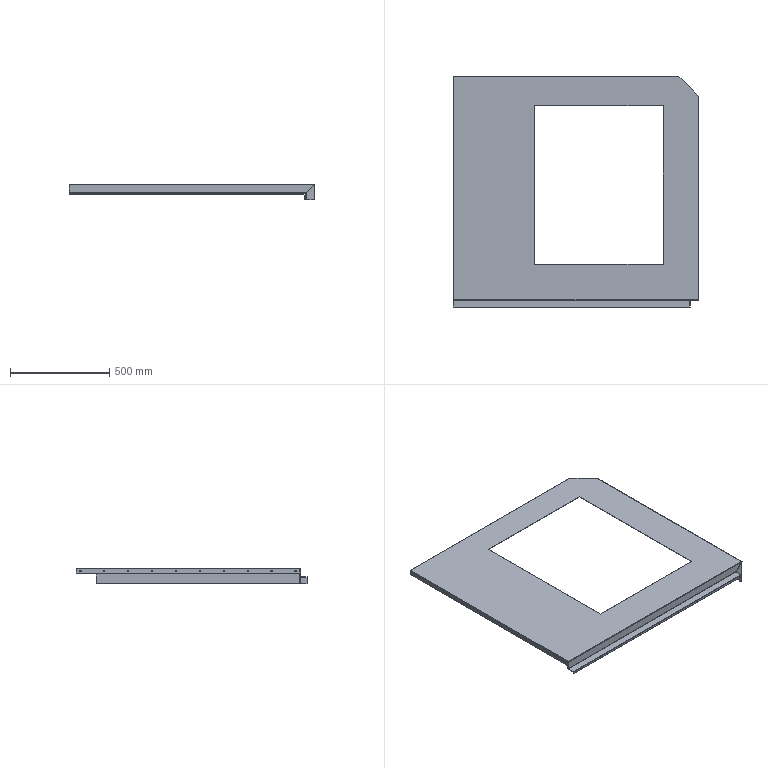Part | STEP file | Left Side Plate | 1 solid | 101 faces | box 1240 x 1166 x 80 mm | volume 2225373 mm3 | plane 54 | cylinder 43 | spline 4 | commonest cylinder face diameters 7 x20 1 x14 5 x9